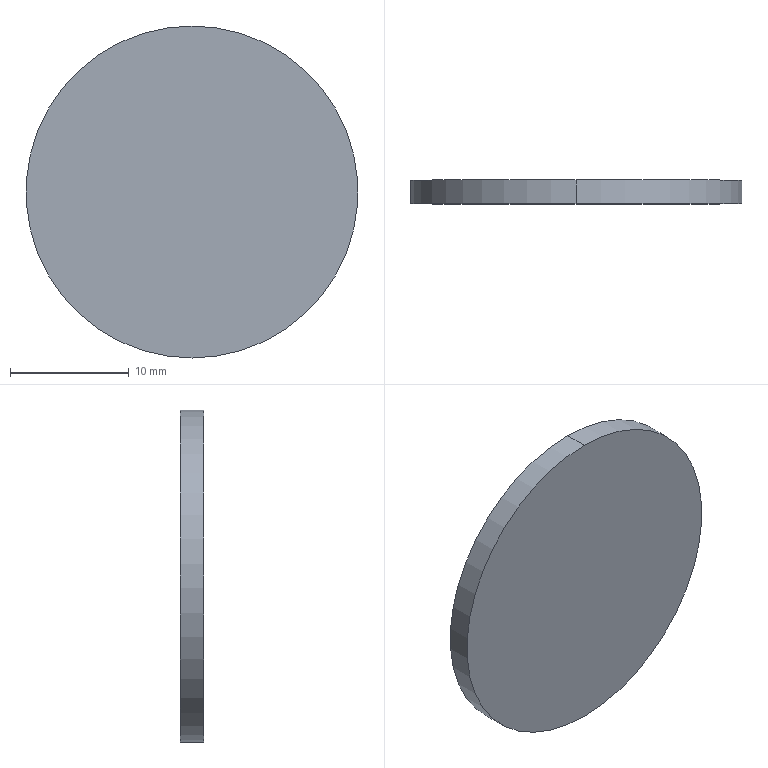Part | SolidWorks | features Extrusion 1 | 1 solid | 4 faces | box 28 x 2 x 28 mm | volume 1232 mm3 | cylinder 2 | plane 2 | commonest cylinder face diameters 28 x2
STEP:
#1=CARTESIAN_POINT('',(0.,2.,14.));
#2=VERTEX_POINT('',#1);
#3=CARTESIAN_POINT('',(0.,2.,-14.));
#4=VERTEX_POINT('',#3);
#5=CARTESIAN_POINT('',(0.,2.,0.));
#6=DIRECTION('',(0.,1.,0.));
#7=DIRECTION('',(0.,0.,1.));
#8=AXIS2_PLACEMENT_3D('',#5,#6,#7);
#9=CIRCLE('',#8,14.);
#10=EDGE_CURVE('',#2,#4,#9,.T.);
#11=ORIENTED_EDGE('',*,*,#10,.F.);
#12=CARTESIAN_POINT('',(0.,0.,14.));
#13=VERTEX_POINT('',#12);
#14=CARTESIAN_POINT('',(0.,2.,14.));
#15=DIRECTION('',(0.,-1.,0.));
#16=VECTOR('',#15,1000.);
#17=LINE('',#14,#16);
#18=EDGE_CURVE('',#2,#13,#17,.T.);
#19=ORIENTED_EDGE('',*,*,#18,.T.);
#20=CARTESIAN_POINT('',(0.,0.,-14.));
#21=VERTEX_POINT('',#20);
#22=CARTESIAN_POINT('',(0.,0.,0.));
#23=DIRECTION('',(0.,1.,0.));
#24=DIRECTION('',(0.,0.,1.));
#25=AXIS2_PLACEMENT_3D('',#22,#23,#24);
#26=CIRCLE('',#25,14.);
#27=EDGE_CURVE('',#13,#21,#26,.T.);
#28=ORIENTED_EDGE('',*,*,#27,.T.);
#29=CARTESIAN_POINT('',(0.,2.,-14.));
#30=DIRECTION('',(0.,-1.,0.));
#31=VECTOR('',#30,1000.);
#32=LINE('',#29,#31);
#33=EDGE_CURVE('',#4,#21,#32,.T.);
#34=ORIENTED_EDGE('',*,*,#33,.F.);
#35=EDGE_LOOP('',(#11,#19,#28,#34));
#36=FACE_OUTER_BOUND('',#35,.T.);
#37=CARTESIAN_POINT('',(0.,2.,0.));
#38=DIRECTION('',(0.,-1.,0.));
#39=DIRECTION('',(0.,0.,-1.));
#40=AXIS2_PLACEMENT_3D('',#37,#38,#39);
#41=CYLINDRICAL_SURFACE('',#40,14.);
#42=ADVANCED_FACE('',(#36),#41,.T.);
#43=ORIENTED_EDGE('',*,*,#18,.F.);
#44=CARTESIAN_POINT('',(0.,2.,0.));
#45=DIRECTION('',(0.,1.,0.));
#46=DIRECTION('',(0.,0.,1.));
#47=AXIS2_PLACEMENT_3D('',#44,#45,#46);
#48=CIRCLE('',#47,14.);
#49=EDGE_CURVE('',#4,#2,#48,.T.);
#50=ORIENTED_EDGE('',*,*,#49,.F.);
#51=ORIENTED_EDGE('',*,*,#33,.T.);
#52=CARTESIAN_POINT('',(0.,0.,0.));
#53=DIRECTION('',(0.,1.,0.));
#54=DIRECTION('',(0.,0.,1.));
#55=AXIS2_PLACEMENT_3D('',#52,#53,#54);
#56=CIRCLE('',#55,14.);
#57=EDGE_CURVE('',#21,#13,#56,.T.);
#58=ORIENTED_EDGE('',*,*,#57,.T.);
#59=EDGE_LOOP('',(#43,#50,#51,#58));
#60=FACE_OUTER_BOUND('',#59,.T.);
#61=CARTESIAN_POINT('',(0.,2.,0.));
#62=DIRECTION('',(0.,-1.,0.));
#63=DIRECTION('',(0.,0.,-1.));
#64=AXIS2_PLACEMENT_3D('',#61,#62,#63);
#65=CYLINDRICAL_SURFACE('',#64,14.);
#66=ADVANCED_FACE('',(#60),#65,.T.);
#67=ORIENTED_EDGE('',*,*,#49,.T.);
#68=ORIENTED_EDGE('',*,*,#10,.T.);
#69=EDGE_LOOP('',(#67,#68));
#70=FACE_OUTER_BOUND('',#69,.T.);
#71=CARTESIAN_POINT('',(0.,2.,0.));
#72=DIRECTION('',(0.,1.,0.));
#73=DIRECTION('',(0.,0.,1.));
#74=AXIS2_PLACEMENT_3D('',#71,#72,#73);
#75=PLANE('',#74);
#76=ADVANCED_FACE('',(#70),#75,.T.);
#77=ORIENTED_EDGE('',*,*,#57,.F.);
#78=ORIENTED_EDGE('',*,*,#27,.F.);
#79=EDGE_LOOP('',(#77,#78));
#80=FACE_OUTER_BOUND('',#79,.T.);
#81=CARTESIAN_POINT('',(0.,0.,0.));
#82=DIRECTION('',(0.,1.,0.));
#83=DIRECTION('',(0.,0.,1.));
#84=AXIS2_PLACEMENT_3D('',#81,#82,#83);
#85=PLANE('',#84);
#86=ADVANCED_FACE('',(#80),#85,.F.);
#87=CLOSED_SHELL('',(#42,#66,#76,#86));
#88=MANIFOLD_SOLID_BREP('',#87);
#89=CARTESIAN_POINT('',(0.,0.,0.));
#90=DIRECTION('',(0.,0.,1.));
#91=DIRECTION('',(1.,0.,0.));
#92=AXIS2_PLACEMENT_3D('',#89,#90,#91);
#93=(LENGTH_UNIT()NAMED_UNIT(*)SI_UNIT(.MILLI.,.METRE.));
#94=UNCERTAINTY_MEASURE_WITH_UNIT(LENGTH_MEASURE(0.00001),#93,'','');
#95=(NAMED_UNIT(*)PLANE_ANGLE_UNIT()SI_UNIT($,.RADIAN.));
#96=(NAMED_UNIT(*)SI_UNIT($,.STERADIAN.)SOLID_ANGLE_UNIT());
#97=(GEOMETRIC_REPRESENTATION_CONTEXT(3)GLOBAL_UNCERTAINTY_ASSIGNED_CONTEXT((#94))GLOBAL_UNIT_ASSIGNED_CONTEXT((#93,#95,#96))REPRESENTATION_CONTEXT('',''));
#98=ADVANCED_BREP_SHAPE_REPRESENTATION('',(#88,#92),#97);